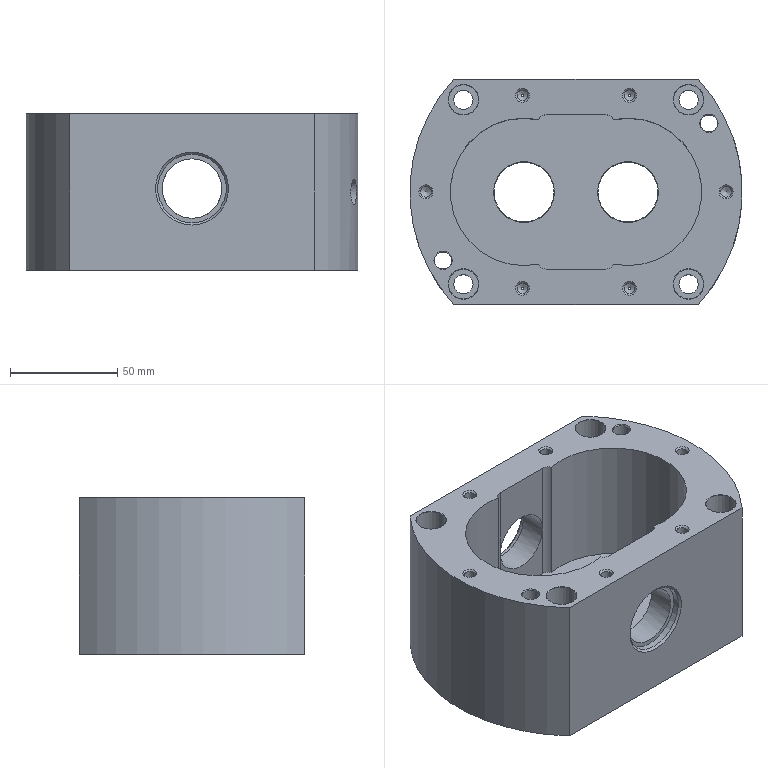NC program | NX | posted with a generic post | part box 155 x 105 x 73.2 mm
Lines 1 to 465 of 30727:
N10 G17 G21 G94 G90
(FLOOR_WALL_COPY_1 , TOOL : D50)
N12 T02 M6
N14 G54
N16 G17 G0 G90 X-115.5 Y62.497 B0. C0. S1200 M3
N18 G43 Z30. H2
N20 Z12.658
N22 G94 G1 Z9.658 F1000.
N24 X-112.5
N26 X112.5 F2000.
N28 Y27.498
N30 X-112.5
N32 Y-7.501
N34 X112.5
N36 Y-42.5
N38 X-112.5
N40 X-115.5
N42 Z12.658
N44 G0 Z30.
N46 Y62.497
N48 Z12.317
N50 G1 Z9.317 F1000.
N52 X-112.5
N54 X112.5 F2000.
N56 Y27.498
N58 X-112.5
N60 Y-7.501
N62 X112.5
N64 Y-42.5
N66 X-112.5
N68 X-115.5
N70 Z12.317
N72 G0 Z30.
N74 Y62.497
N76 Z11.976
N78 G1 Z8.976 F1000.
N80 X-112.5
N82 X112.5 F2000.
N84 Y27.498
N86 X-112.5
N88 Y-7.501
N90 X112.5
N92 Y-42.5
N94 X-112.5
N96 X-115.5
N98 Z11.976
N100 G0 Z30.
N102 Y62.497
N104 Z11.634
N106 G1 Z8.634 F1000.
N108 X-112.5
N110 X112.5 F2000.
N112 Y27.498
N114 X-112.5
N116 Y-7.501
N118 X112.5
N120 Y-42.5
N122 X-112.5
N124 X-115.5
N126 Z11.634
N128 G0 Z30.
N130 Y62.497
N132 Z11.293
N134 G1 Z8.293 F1000.
N136 X-112.5
N138 X112.5 F2000.
N140 Y27.498
N142 X-112.5
N144 Y-7.501
N146 X112.5
N148 Y-42.5
N150 X-112.5
N152 X-115.5
N154 Z11.293
N156 G0 Z30.
N158 Y62.497
N160 Z10.951
N162 G1 Z7.951 F1000.
N164 X-112.5
N166 X112.5 F2000.
N168 Y27.498
N170 X-112.5
N172 Y-7.501
N174 X112.5
N176 Y-42.5
N178 X-112.5
N180 X-115.5
N182 Z10.951
N184 G0 Z30.
N186 Y62.497
N188 Z10.61
N190 G1 Z7.61 F1000.
N192 X-112.5
N194 X112.5 F2000.
N196 Y27.498
N198 X-112.5
N200 Y-7.501
N202 X112.5
N204 Y-42.5
N206 X-112.5
N208 X-115.5
N210 Z10.61
N212 G0 Z30.
N214 Y62.497
N216 Z10.269
N218 G1 Z7.269 F1000.
N220 X-112.5
N222 X112.5 F2000.
N224 Y27.498
N226 X-112.5
N228 Y-7.501
N230 X112.5
N232 Y-42.5
N234 X-112.5
N236 X-115.5
N238 Z10.269
N240 G0 Z30.
N242 Y62.497
N244 Z9.927
N246 G1 Z6.927 F1000.
N248 X-112.5
N250 X112.5 F2000.
N252 Y27.498
N254 X-112.5
N256 Y-7.501
N258 X112.5
N260 Y-42.5
N262 X-112.5
N264 X-115.5
N266 Z9.927
N268 G0 Z30.
N270 Y62.497
N272 Z9.586
N274 G1 Z6.586 F1000.
N276 X-112.5
N278 X112.5 F2000.
N280 Y27.498
N282 X-112.5
N284 Y-7.501
N286 X112.5
N288 Y-42.5
N290 X-112.5
N292 X-115.5
N294 Z9.586
N296 G0 Z30.
N298 Y62.497
N300 Z9.245
N302 G1 Z6.245 F1000.
N304 X-112.5
N306 X112.5 F2000.
N308 Y27.498
N310 X-112.5
N312 Y-7.501
N314 X112.5
N316 Y-42.5
N318 X-112.5
N320 X-115.5
N322 Z9.245
N324 G0 Z30.
N326 Y62.497
N328 Z8.903
N330 G1 Z5.903 F1000.
N332 X-112.5
N334 X112.5 F2000.
N336 Y27.498
N338 X-112.5
N340 Y-7.501
N342 X112.5
N344 Y-42.5
N346 X-112.5
N348 X-115.5
N350 Z8.903
N352 G0 Z30.
N354 Y62.497
N356 Z8.562
N358 G1 Z5.562 F1000.
N360 X-112.5
N362 X112.5 F2000.
N364 Y27.498
N366 X-112.5
N368 Y-7.501
N370 X112.5
N372 Y-42.5
N374 X-112.5
N376 X-115.5
N378 Z8.562
N380 G0 Z30.
N382 Y62.497
N384 Z8.221
N386 G1 Z5.221 F1000.
N388 X-112.5
N390 X112.5 F2000.
N392 Y27.498
N394 X-112.5
N396 Y-7.501
N398 X112.5
N400 Y-42.5
N402 X-112.5
N404 X-115.5
N406 Z8.221
N408 G0 Z30.
N410 Y62.497
N412 Z7.879
N414 G1 Z4.879 F1000.
N416 X-112.5
N418 X112.5 F2000.
N420 Y27.498
N422 X-112.5
N424 Y-7.501
N426 X112.5
N428 Y-42.5
N430 X-112.5
N432 X-115.5
N434 Z7.879
N436 G0 Z30.
N438 Y62.497
N440 Z7.538
N442 G1 Z4.538 F1000.
N444 X-112.5
N446 X112.5 F2000.
N448 Y27.498
N450 X-112.5
N452 Y-7.501
N454 X112.5
N456 Y-42.5
N458 X-112.5
N460 X-115.5
N462 Z7.538
N464 G0 Z30.
N466 Y62.497
N468 Z7.196
N470 G1 Z4.196 F1000.
N472 X-112.5
N474 X112.5 F2000.
N476 Y27.498
N478 X-112.5
N480 Y-7.501
N482 X112.5
N484 Y-42.5
N486 X-112.5
N488 X-115.5
N490 Z7.196
N492 G0 Z30.
N494 Y62.497
N496 Z6.855
N498 G1 Z3.855 F1000.
N500 X-112.5
N502 X112.5 F2000.
N504 Y27.498
N506 X-112.5
N508 Y-7.501
N510 X112.5
N512 Y-42.5
N514 X-112.5
N516 X-115.5
N518 Z6.855
N520 G0 Z30.
N522 Y62.497
N524 Z6.514
N526 G1 Z3.514 F1000.
N528 X-112.5
N530 X112.5 F2000.
N532 Y27.498
N534 X-112.5
N536 Y-7.501
N538 X112.5
N540 Y-42.5
N542 X-112.5
N544 X-115.5
N546 Z6.514
N548 G0 Z30.
N550 Y62.497
N552 Z6.172
N554 G1 Z3.172 F1000.
N556 X-112.5
N558 X112.5 F2000.
N560 Y27.498
N562 X-112.5
N564 Y-7.501
N566 X112.5
N568 Y-42.5
N570 X-112.5
N572 X-115.5
N574 Z6.172
N576 G0 Z30.
N578 Y62.497
N580 Z5.831
N582 G1 Z2.831 F1000.
N584 X-112.5
N586 X112.5 F2000.
N588 Y27.498
N590 X-112.5
N592 Y-7.501
N594 X112.5
N596 Y-42.5
N598 X-112.5
N600 X-115.5
N602 Z5.831
N604 G0 Z30.
N606 Y62.497
N608 Z5.49
N610 G1 Z2.49 F1000.
N612 X-112.5
N614 X112.5 F2000.
N616 Y27.498
N618 X-112.5
N620 Y-7.501
N622 X112.5
N624 Y-42.5
N626 X-112.5
N628 X-115.5
N630 Z5.49
N632 G0 Z30.
N634 Y62.497
N636 Z5.148
N638 G1 Z2.148 F1000.
N640 X-112.5
N642 X112.5 F2000.
N644 Y27.498
N646 X-112.5
N648 Y-7.501
N650 X112.5
N652 Y-42.5
N654 X-112.5
N656 X-115.5
N658 Z5.148
N660 G0 Z30.
N662 Y62.497
N664 Z4.807
N666 G1 Z1.807 F1000.
N668 X-112.5
N670 X112.5 F2000.
N672 Y27.498
N674 X-112.5
N676 Y-7.501
N678 X112.5
N680 Y-42.5
N682 X-112.5
N684 X-115.5
N686 Z4.807
N688 G0 Z30.
N690 Y62.497
N692 Z4.465
N694 G1 Z1.465 F1000.
N696 X-112.5
N698 X112.5 F2000.
N700 Y27.498
N702 X-112.5
N704 Y-7.501
N706 X112.5
N708 Y-42.5
N710 X-112.5
N712 X-115.5
N714 Z4.465
N716 G0 Z30.
N718 Y62.497
N720 Z4.124
N722 G1 Z1.124 F1000.
N724 X-112.5
N726 X112.5 F2000.
N728 Y27.498
N730 X-112.5
N732 Y-7.501
N734 X112.5
N736 Y-42.5
N738 X-112.5
N740 X-115.5
N742 Z4.124
N744 G0 Z30.
N746 Y62.497
N748 Z3.783
N750 G1 Z0.783 F1000.
N752 X-112.5
N754 X112.5 F2000.
N756 Y27.498
N758 X-112.5
N760 Y-7.501
N762 X112.5
N764 Y-42.5
N766 X-112.5
N768 X-115.5
N770 Z3.783
N772 G0 Z30.
N774 Y62.497
N776 Z3.441
N778 G1 Z0.441 F1000.
N780 X-112.5
N782 X112.5 F2000.
N784 Y27.498
N786 X-112.5
N788 Y-7.501
N790 X112.5
N792 Y-42.5
N794 X-112.5
N796 X-115.5
N798 Z3.441
N800 G0 Z30.
N802 Y62.497
N804 Z3.1
N806 G1 Z0.1 F1000.
N808 X-112.5
N810 X112.5 F2000.
N812 Y27.498
N814 X-112.5
N816 Y-7.501
N818 X112.5
N820 Y-42.5
N822 X-112.5
N824 X-115.5
N826 Z3.1
N828 G0 Z30.
(FLOOR_WALL_COPY_COPY , TOOL : D50)
N830 Y62.497 S2500
N832 Z3.
N834 G1 Z0. F1000.
N836 X-112.5
N838 X112.5
N840 Y27.498
N842 X-112.5
N844 Y-7.501
N846 X112.5
N848 Y-42.5
N850 X-112.5
N852 X-115.5
N854 Z3.
N856 G0 Z30.
N858 M5
(DRILLING_COPY_1 , TOOL : ZXZ)
N860 T01 M6
N862 G54
N864 G17 G0 G90 X-70. Y0. B0. C0. S5000 M3
N866 G43 Z30. H1
N868 G94 G81 G98 Z-1. F250. R3.
N870 X-25. Y45.
N872 X25.
N874 X70. Y0.
N876 X25. Y-45.
N878 X-25.
N880 G80
N882 G0 X-25. Y-45. Z30.
N884 M5
(DRILLING_COPY_1_COPY , TOOL : 5.0ZT)
N886 T15 M6
N888 G54
N890 G17 G0 G90 X-70. Y0. B0. C0. S2000 M3
N892 G43 Z30. H15
N894 G94 G83 G98 Z-24.502 F200. Q2. R3.
N896 X-25. Y45.
N898 X25.
N900 X70. Y0.
N902 X25. Y-45.
N904 X-25.
N906 G80
N908 G0 X-25. Y-45. Z30.
N910 M5